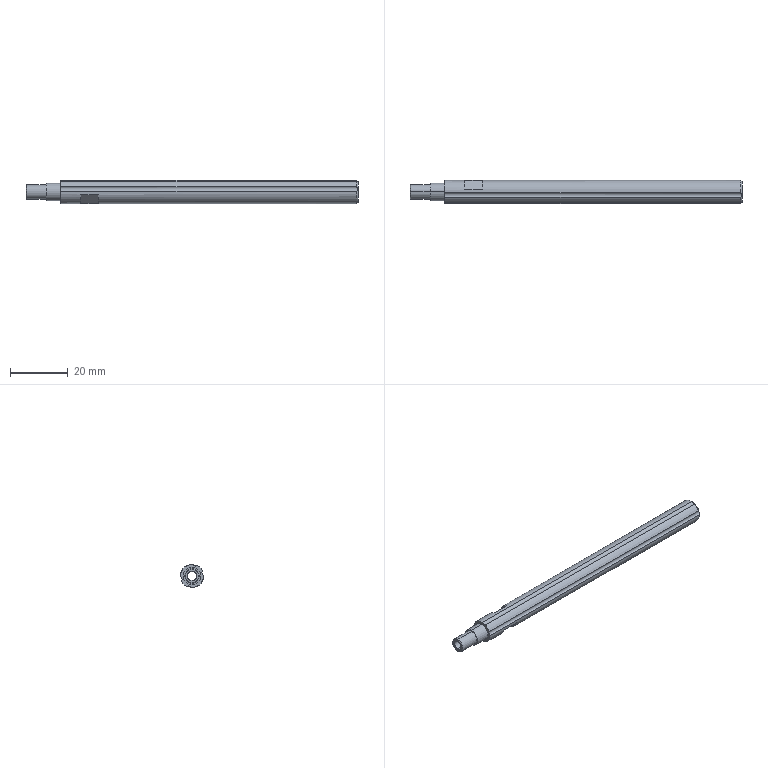Part | SolidWorks | features ICE 3, Chamfer 2, BaseBody 1, MoveFace 1 | 1 solid | 30 faces | box 115 x 8 x 8 mm | volume 4454 mm3 | cylinder 14 | plane 10 | cone 6 | commonest cylinder face diameters 2.08 x4 8 x4 3 x2 5 x2 6 x2
STEP:
#1=CARTESIAN_POINT('',(115.,0.,-3.5));
#2=VERTEX_POINT('',#1);
#3=CARTESIAN_POINT('',(115.,0.,3.5));
#4=VERTEX_POINT('',#3);
#5=CARTESIAN_POINT('',(115.,0.,0.));
#6=DIRECTION('',(1.,0.,0.));
#7=DIRECTION('',(0.,0.,-1.));
#8=AXIS2_PLACEMENT_3D('',#5,#6,#7);
#9=CIRCLE('',#8,3.5);
#10=EDGE_CURVE('',#2,#4,#9,.T.);
#11=ORIENTED_EDGE('',*,*,#10,.F.);
#12=CARTESIAN_POINT('',(114.5,0.,-4.));
#13=VERTEX_POINT('',#12);
#14=CARTESIAN_POINT('',(115.,0.,-3.5));
#15=DIRECTION('',(-0.7071,0.,-0.7071));
#16=VECTOR('',#15,1000.);
#17=LINE('',#14,#16);
#18=EDGE_CURVE('',#2,#13,#17,.T.);
#19=ORIENTED_EDGE('',*,*,#18,.T.);
#20=CARTESIAN_POINT('',(114.5,0.2928,-3.989));
#21=VERTEX_POINT('',#20);
#22=CARTESIAN_POINT('',(114.5,0.,0.));
#23=DIRECTION('',(-1.,0.,0.));
#24=DIRECTION('',(0.,0.,1.));
#25=AXIS2_PLACEMENT_3D('',#22,#23,#24);
#26=CIRCLE('',#25,4.);
#27=EDGE_CURVE('',#21,#13,#26,.T.);
#28=ORIENTED_EDGE('',*,*,#27,.F.);
#29=CARTESIAN_POINT('',(114.5,1.741,-3.601));
#30=VERTEX_POINT('',#29);
#31=CARTESIAN_POINT('',(114.5,1.741,-3.601));
#32=CARTESIAN_POINT('',(114.601,1.638,-3.539));
#33=CARTESIAN_POINT('',(114.695,1.519,-3.491));
#34=CARTESIAN_POINT('',(114.841,1.245,-3.443));
#35=CARTESIAN_POINT('',(114.89,1.087,-3.446));
#36=CARTESIAN_POINT('',(114.89,0.7827,-3.528));
#37=CARTESIAN_POINT('',(114.841,0.6442,-3.604));
#38=CARTESIAN_POINT('',(114.695,0.4305,-3.782));
#39=CARTESIAN_POINT('',(114.601,0.3513,-3.883));
#40=CARTESIAN_POINT('',(114.5,0.2928,-3.989));
#41=B_SPLINE_CURVE_WITH_KNOTS('',3,(#31,#32,#33,#34,#35,#36,#37,#38,#39,#40),.UNSPECIFIED.,.F.,.F.,(4,2,2,2,4),(0.,0.0004682,0.0009363,0.001404,0.001873),.UNSPECIFIED.);
#42=EDGE_CURVE('',#30,#21,#41,.T.);
#43=ORIENTED_EDGE('',*,*,#42,.F.);
#44=CARTESIAN_POINT('',(114.5,3.601,-1.741));
#45=VERTEX_POINT('',#44);
#46=CARTESIAN_POINT('',(114.5,0.,0.));
#47=DIRECTION('',(-1.,0.,0.));
#48=DIRECTION('',(0.,0.,1.));
#49=AXIS2_PLACEMENT_3D('',#46,#47,#48);
#50=CIRCLE('',#49,4.);
#51=EDGE_CURVE('',#45,#30,#50,.T.);
#52=ORIENTED_EDGE('',*,*,#51,.F.);
#53=CARTESIAN_POINT('',(114.5,3.989,-0.2928));
#54=VERTEX_POINT('',#53);
#55=CARTESIAN_POINT('',(114.5,3.989,-0.2928));
#56=CARTESIAN_POINT('',(114.601,3.883,-0.3512));
#57=CARTESIAN_POINT('',(114.695,3.783,-0.43));
#58=CARTESIAN_POINT('',(114.841,3.604,-0.6436));
#59=CARTESIAN_POINT('',(114.89,3.528,-0.7816));
#60=CARTESIAN_POINT('',(114.89,3.446,-1.086));
#61=CARTESIAN_POINT('',(114.841,3.443,-1.244));
#62=CARTESIAN_POINT('',(114.695,3.491,-1.518));
#63=CARTESIAN_POINT('',(114.601,3.539,-1.637));
#64=CARTESIAN_POINT('',(114.5,3.601,-1.741));
#65=B_SPLINE_CURVE_WITH_KNOTS('',3,(#55,#56,#57,#58,#59,#60,#61,#62,#63,#64),.UNSPECIFIED.,.F.,.F.,(4,2,2,2,4),(0.,0.0004682,0.0009363,0.001404,0.001873),.UNSPECIFIED.);
#66=EDGE_CURVE('',#54,#45,#65,.T.);
#67=ORIENTED_EDGE('',*,*,#66,.F.);
#68=CARTESIAN_POINT('',(114.5,0.,4.));
#69=VERTEX_POINT('',#68);
#70=CARTESIAN_POINT('',(114.5,0.,0.));
#71=DIRECTION('',(-1.,0.,0.));
#72=DIRECTION('',(0.,0.,1.));
#73=AXIS2_PLACEMENT_3D('',#70,#71,#72);
#74=CIRCLE('',#73,4.);
#75=EDGE_CURVE('',#69,#54,#74,.T.);
#76=ORIENTED_EDGE('',*,*,#75,.F.);
#77=CARTESIAN_POINT('',(115.,0.,3.5));
#78=DIRECTION('',(-0.7071,0.,0.7071));
#79=VECTOR('',#78,1000.);
#80=LINE('',#77,#79);
#81=EDGE_CURVE('',#4,#69,#80,.T.);
#82=ORIENTED_EDGE('',*,*,#81,.F.);
#83=EDGE_LOOP('',(#11,#19,#28,#43,#52,#67,#76,#82));
#84=FACE_OUTER_BOUND('',#83,.T.);
#85=CARTESIAN_POINT('',(115.,0.,0.));
#86=DIRECTION('',(-1.,0.,0.));
#87=DIRECTION('',(0.,0.,1.));
#88=AXIS2_PLACEMENT_3D('',#85,#86,#87);
#89=CONICAL_SURFACE('',#88,3.5,0.7854);
#90=ADVANCED_FACE('',(#84),#89,.T.);
#91=CARTESIAN_POINT('',(0.,0.,2.3));
#92=VERTEX_POINT('',#91);
#93=CARTESIAN_POINT('',(0.,0.,-2.3));
#94=VERTEX_POINT('',#93);
#95=CARTESIAN_POINT('',(0.,0.,0.));
#96=DIRECTION('',(-1.,0.,0.));
#97=DIRECTION('',(0.,0.,-1.));
#98=AXIS2_PLACEMENT_3D('',#95,#96,#97);
#99=CIRCLE('',#98,2.3);
#100=EDGE_CURVE('',#92,#94,#99,.T.);
#101=ORIENTED_EDGE('',*,*,#100,.F.);
#102=CARTESIAN_POINT('',(0.2,0.,2.5));
#103=VERTEX_POINT('',#102);
#104=CARTESIAN_POINT('',(0.,0.,2.3));
#105=DIRECTION('',(0.7071,0.,0.7071));
#106=VECTOR('',#105,1000.);
#107=LINE('',#104,#106);
#108=EDGE_CURVE('',#92,#103,#107,.T.);
#109=ORIENTED_EDGE('',*,*,#108,.T.);
#110=CARTESIAN_POINT('',(0.2,0.,-2.5));
#111=VERTEX_POINT('',#110);
#112=CARTESIAN_POINT('',(0.2,0.,0.));
#113=DIRECTION('',(1.,0.,0.));
#114=DIRECTION('',(0.,0.,-1.));
#115=AXIS2_PLACEMENT_3D('',#112,#113,#114);
#116=CIRCLE('',#115,2.5);
#117=EDGE_CURVE('',#111,#103,#116,.T.);
#118=ORIENTED_EDGE('',*,*,#117,.F.);
#119=CARTESIAN_POINT('',(0.,0.,-2.3));
#120=DIRECTION('',(0.7071,0.,-0.7071));
#121=VECTOR('',#120,1000.);
#122=LINE('',#119,#121);
#123=EDGE_CURVE('',#94,#111,#122,.T.);
#124=ORIENTED_EDGE('',*,*,#123,.F.);
#125=EDGE_LOOP('',(#101,#109,#118,#124));
#126=FACE_OUTER_BOUND('',#125,.T.);
#127=CARTESIAN_POINT('',(0.,0.,0.));
#128=DIRECTION('',(1.,0.,0.));
#129=DIRECTION('',(0.,0.,-1.));
#130=AXIS2_PLACEMENT_3D('',#127,#128,#129);
#131=CONICAL_SURFACE('',#130,2.3,0.7854);
#132=ADVANCED_FACE('',(#126),#131,.T.);
#133=CARTESIAN_POINT('',(7.,0.,2.5));
#134=VERTEX_POINT('',#133);
#135=CARTESIAN_POINT('',(7.,0.,-2.5));
#136=VERTEX_POINT('',#135);
#137=CARTESIAN_POINT('',(7.,0.,0.));
#138=DIRECTION('',(-1.,0.,0.));
#139=DIRECTION('',(0.,0.,1.));
#140=AXIS2_PLACEMENT_3D('',#137,#138,#139);
#141=CIRCLE('',#140,2.5);
#142=EDGE_CURVE('',#134,#136,#141,.T.);
#143=ORIENTED_EDGE('',*,*,#142,.T.);
#144=CARTESIAN_POINT('',(7.,0.,-2.5));
#145=DIRECTION('',(-1.,0.,0.));
#146=VECTOR('',#145,1000.);
#147=LINE('',#144,#146);
#148=EDGE_CURVE('',#136,#111,#147,.T.);
#149=ORIENTED_EDGE('',*,*,#148,.T.);
#150=ORIENTED_EDGE('',*,*,#117,.T.);
#151=CARTESIAN_POINT('',(7.,0.,2.5));
#152=DIRECTION('',(-1.,0.,0.));
#153=VECTOR('',#152,1000.);
#154=LINE('',#151,#153);
#155=EDGE_CURVE('',#134,#103,#154,.T.);
#156=ORIENTED_EDGE('',*,*,#155,.F.);
#157=EDGE_LOOP('',(#143,#149,#150,#156));
#158=FACE_OUTER_BOUND('',#157,.T.);
#159=CARTESIAN_POINT('',(7.,0.,0.));
#160=DIRECTION('',(-1.,0.,0.));
#161=DIRECTION('',(0.,0.,1.));
#162=AXIS2_PLACEMENT_3D('',#159,#160,#161);
#163=CYLINDRICAL_SURFACE('',#162,2.5);
#164=ADVANCED_FACE('',(#158),#163,.T.);
#165=CARTESIAN_POINT('',(12.,0.,3.));
#166=VERTEX_POINT('',#165);
#167=CARTESIAN_POINT('',(12.,0.,-3.));
#168=VERTEX_POINT('',#167);
#169=CARTESIAN_POINT('',(12.,0.,0.));
#170=DIRECTION('',(-1.,0.,0.));
#171=DIRECTION('',(0.,0.,1.));
#172=AXIS2_PLACEMENT_3D('',#169,#170,#171);
#173=CIRCLE('',#172,3.);
#174=EDGE_CURVE('',#166,#168,#173,.T.);
#175=ORIENTED_EDGE('',*,*,#174,.T.);
#176=CARTESIAN_POINT('',(7.,0.,-3.));
#177=VERTEX_POINT('',#176);
#178=CARTESIAN_POINT('',(12.,0.,-3.));
#179=DIRECTION('',(-1.,0.,0.));
#180=VECTOR('',#179,1000.);
#181=LINE('',#178,#180);
#182=EDGE_CURVE('',#168,#177,#181,.T.);
#183=ORIENTED_EDGE('',*,*,#182,.T.);
#184=CARTESIAN_POINT('',(7.,0.,3.));
#185=VERTEX_POINT('',#184);
#186=CARTESIAN_POINT('',(7.,0.,0.));
#187=DIRECTION('',(1.,0.,0.));
#188=DIRECTION('',(0.,0.,1.));
#189=AXIS2_PLACEMENT_3D('',#186,#187,#188);
#190=CIRCLE('',#189,3.);
#191=EDGE_CURVE('',#177,#185,#190,.T.);
#192=ORIENTED_EDGE('',*,*,#191,.T.);
#193=CARTESIAN_POINT('',(12.,0.,3.));
#194=DIRECTION('',(-1.,0.,0.));
#195=VECTOR('',#194,1000.);
#196=LINE('',#193,#195);
#197=EDGE_CURVE('',#166,#185,#196,.T.);
#198=ORIENTED_EDGE('',*,*,#197,.F.);
#199=EDGE_LOOP('',(#175,#183,#192,#198));
#200=FACE_OUTER_BOUND('',#199,.T.);
#201=CARTESIAN_POINT('',(12.,0.,0.));
#202=DIRECTION('',(-1.,0.,0.));
#203=DIRECTION('',(0.,0.,1.));
#204=AXIS2_PLACEMENT_3D('',#201,#202,#203);
#205=CYLINDRICAL_SURFACE('',#204,3.);
#206=ADVANCED_FACE('',(#200),#205,.T.);
#207=CARTESIAN_POINT('',(12.,0.2928,-3.989));
#208=VERTEX_POINT('',#207);
#209=CARTESIAN_POINT('',(90.,0.2928,-3.989));
#210=DIRECTION('',(-1.,0.,0.));
#211=VECTOR('',#210,1000.);
#212=LINE('',#209,#211);
#213=EDGE_CURVE('',#21,#208,#212,.T.);
#214=ORIENTED_EDGE('',*,*,#213,.F.);
#215=ORIENTED_EDGE('',*,*,#27,.T.);
#216=CARTESIAN_POINT('',(114.5,-3.989,0.2928));
#217=VERTEX_POINT('',#216);
#218=CARTESIAN_POINT('',(114.5,0.,0.));
#219=DIRECTION('',(-1.,0.,0.));
#220=DIRECTION('',(0.,0.,1.));
#221=AXIS2_PLACEMENT_3D('',#218,#219,#220);
#222=CIRCLE('',#221,4.);
#223=EDGE_CURVE('',#13,#217,#222,.T.);
#224=ORIENTED_EDGE('',*,*,#223,.T.);
#225=CARTESIAN_POINT('',(12.,-3.989,0.2928));
#226=VERTEX_POINT('',#225);
#227=CARTESIAN_POINT('',(90.,-3.989,0.2928));
#228=DIRECTION('',(-1.,0.,0.));
#229=VECTOR('',#228,1000.);
#230=LINE('',#227,#229);
#231=EDGE_CURVE('',#217,#226,#230,.T.);
#232=ORIENTED_EDGE('',*,*,#231,.T.);
#233=CARTESIAN_POINT('',(12.,0.,0.));
#234=DIRECTION('',(1.,0.,0.));
#235=DIRECTION('',(0.,0.,1.));
#236=AXIS2_PLACEMENT_3D('',#233,#234,#235);
#237=CIRCLE('',#236,4.);
#238=EDGE_CURVE('',#226,#208,#237,.T.);
#239=ORIENTED_EDGE('',*,*,#238,.T.);
#240=EDGE_LOOP('',(#214,#215,#224,#232,#239));
#241=FACE_OUTER_BOUND('',#240,.T.);
#242=CARTESIAN_POINT('',(19.,-0.9142,-3.894));
#243=VERTEX_POINT('',#242);
#244=CARTESIAN_POINT('',(25.,-0.9142,-3.894));
#245=VERTEX_POINT('',#244);
#246=CARTESIAN_POINT('',(90.,-0.9142,-3.894));
#247=DIRECTION('',(1.,0.,0.));
#248=VECTOR('',#247,1000.);
#249=LINE('',#246,#248);
#250=EDGE_CURVE('',#243,#245,#249,.T.);
#251=ORIENTED_EDGE('',*,*,#250,.F.);
#252=CARTESIAN_POINT('',(19.,-3.894,-0.9142));
#253=VERTEX_POINT('',#252);
#254=CARTESIAN_POINT('',(19.,0.,0.));
#255=DIRECTION('',(-1.,0.,0.));
#256=DIRECTION('',(0.,0.,-1.));
#257=AXIS2_PLACEMENT_3D('',#254,#255,#256);
#258=CIRCLE('',#257,4.);
#259=EDGE_CURVE('',#243,#253,#258,.T.);
#260=ORIENTED_EDGE('',*,*,#259,.T.);
#261=CARTESIAN_POINT('',(25.,-3.894,-0.9142));
#262=VERTEX_POINT('',#261);
#263=CARTESIAN_POINT('',(90.,-3.894,-0.9142));
#264=DIRECTION('',(-1.,0.,0.));
#265=VECTOR('',#264,1000.);
#266=LINE('',#263,#265);
#267=EDGE_CURVE('',#262,#253,#266,.T.);
#268=ORIENTED_EDGE('',*,*,#267,.F.);
#269=CARTESIAN_POINT('',(25.,0.,0.));
#270=DIRECTION('',(-1.,0.,0.));
#271=DIRECTION('',(0.,0.,-1.));
#272=AXIS2_PLACEMENT_3D('',#269,#270,#271);
#273=CIRCLE('',#272,4.);
#274=EDGE_CURVE('',#245,#262,#273,.T.);
#275=ORIENTED_EDGE('',*,*,#274,.F.);
#276=EDGE_LOOP('',(#251,#260,#268,#275));
#277=FACE_BOUND('',#276,.T.);
#278=CARTESIAN_POINT('',(90.,0.,0.));
#279=DIRECTION('',(-1.,0.,0.));
#280=DIRECTION('',(0.,0.7071,0.7071));
#281=AXIS2_PLACEMENT_3D('',#278,#279,#280);
#282=CYLINDRICAL_SURFACE('',#281,4.);
#283=ADVANCED_FACE('',(#241,#277),#282,.T.);
#284=CARTESIAN_POINT('',(114.5,-0.2928,3.989));
#285=VERTEX_POINT('',#284);
#286=CARTESIAN_POINT('',(12.,-0.2928,3.989));
#287=VERTEX_POINT('',#286);
#288=CARTESIAN_POINT('',(90.,-0.2928,3.989));
#289=DIRECTION('',(-1.,0.,0.));
#290=VECTOR('',#289,1000.);
#291=LINE('',#288,#290);
#292=EDGE_CURVE('',#285,#287,#291,.T.);
#293=ORIENTED_EDGE('',*,*,#292,.F.);
#294=CARTESIAN_POINT('',(114.5,0.,0.));
#295=DIRECTION('',(-1.,0.,0.));
#296=DIRECTION('',(0.,0.,1.));
#297=AXIS2_PLACEMENT_3D('',#294,#295,#296);
#298=CIRCLE('',#297,4.);
#299=EDGE_CURVE('',#285,#69,#298,.T.);
#300=ORIENTED_EDGE('',*,*,#299,.T.);
#301=ORIENTED_EDGE('',*,*,#75,.T.);
#302=CARTESIAN_POINT('',(12.,3.989,-0.2928));
#303=VERTEX_POINT('',#302);
#304=CARTESIAN_POINT('',(90.,3.989,-0.2928));
#305=DIRECTION('',(-1.,0.,0.));
#306=VECTOR('',#305,1000.);
#307=LINE('',#304,#306);
#308=EDGE_CURVE('',#54,#303,#307,.T.);
#309=ORIENTED_EDGE('',*,*,#308,.T.);
#310=CARTESIAN_POINT('',(12.,0.,0.));
#311=DIRECTION('',(1.,0.,0.));
#312=DIRECTION('',(0.,0.,1.));
#313=AXIS2_PLACEMENT_3D('',#310,#311,#312);
#314=CIRCLE('',#313,4.);
#315=EDGE_CURVE('',#303,#287,#314,.T.);
#316=ORIENTED_EDGE('',*,*,#315,.T.);
#317=EDGE_LOOP('',(#293,#300,#301,#309,#316));
#318=FACE_OUTER_BOUND('',#317,.T.);
#319=CARTESIAN_POINT('',(19.,0.9142,3.894));
#320=VERTEX_POINT('',#319);
#321=CARTESIAN_POINT('',(25.,0.9142,3.894));
#322=VERTEX_POINT('',#321);
#323=CARTESIAN_POINT('',(90.,0.9142,3.894));
#324=DIRECTION('',(1.,0.,0.));
#325=VECTOR('',#324,1000.);
#326=LINE('',#323,#325);
#327=EDGE_CURVE('',#320,#322,#326,.T.);
#328=ORIENTED_EDGE('',*,*,#327,.F.);
#329=CARTESIAN_POINT('',(19.,3.894,0.9142));
#330=VERTEX_POINT('',#329);
#331=CARTESIAN_POINT('',(19.,0.,0.));
#332=DIRECTION('',(-1.,0.,0.));
#333=DIRECTION('',(0.,0.,-1.));
#334=AXIS2_PLACEMENT_3D('',#331,#332,#333);
#335=CIRCLE('',#334,4.);
#336=EDGE_CURVE('',#320,#330,#335,.T.);
#337=ORIENTED_EDGE('',*,*,#336,.T.);
#338=CARTESIAN_POINT('',(25.,3.894,0.9142));
#339=VERTEX_POINT('',#338);
#340=CARTESIAN_POINT('',(90.,3.894,0.9142));
#341=DIRECTION('',(-1.,0.,0.));
#342=VECTOR('',#341,1000.);
#343=LINE('',#340,#342);
#344=EDGE_CURVE('',#339,#330,#343,.T.);
#345=ORIENTED_EDGE('',*,*,#344,.F.);
#346=CARTESIAN_POINT('',(25.,0.,0.));
#347=DIRECTION('',(-1.,0.,0.));
#348=DIRECTION('',(0.,0.,-1.));
#349=AXIS2_PLACEMENT_3D('',#346,#347,#348);
#350=CIRCLE('',#349,4.);
#351=EDGE_CURVE('',#322,#339,#350,.T.);
#352=ORIENTED_EDGE('',*,*,#351,.F.);
#353=EDGE_LOOP('',(#328,#337,#345,#352));
#354=FACE_BOUND('',#353,.T.);
#355=CARTESIAN_POINT('',(90.,0.,0.));
#356=DIRECTION('',(-1.,0.,0.));
#357=DIRECTION('',(0.,-0.7071,-0.7071));
#358=AXIS2_PLACEMENT_3D('',#355,#356,#357);
#359=CYLINDRICAL_SURFACE('',#358,4.);
#360=ADVANCED_FACE('',(#318,#354),#359,.T.);
#361=CARTESIAN_POINT('',(0.,0.,-1.7));
#362=VERTEX_POINT('',#361);
#363=CARTESIAN_POINT('',(0.,0.,1.7));
#364=VERTEX_POINT('',#363);
#365=CARTESIAN_POINT('',(0.,0.,0.));
#366=DIRECTION('',(1.,0.,0.));
#367=DIRECTION('',(0.,0.,-1.));
#368=AXIS2_PLACEMENT_3D('',#365,#366,#367);
#369=CIRCLE('',#368,1.7);
#370=EDGE_CURVE('',#362,#364,#369,.T.);
#371=ORIENTED_EDGE('',*,*,#370,.T.);
#372=CARTESIAN_POINT('',(0.,0.,0.));
#373=DIRECTION('',(1.,0.,0.));
#374=DIRECTION('',(0.,0.,-1.));
#375=AXIS2_PLACEMENT_3D('',#372,#373,#374);
#376=CIRCLE('',#375,1.7);
#377=EDGE_CURVE('',#364,#362,#376,.T.);
#378=ORIENTED_EDGE('',*,*,#377,.T.);
#379=EDGE_LOOP('',(#371,#378));
#380=FACE_BOUND('',#379,.T.);
#381=CARTESIAN_POINT('',(0.,0.,0.));
#382=DIRECTION('',(-1.,0.,0.));
#383=DIRECTION('',(0.,0.,-1.));
#384=AXIS2_PLACEMENT_3D('',#381,#382,#383);
#385=CIRCLE('',#384,2.3);
#386=EDGE_CURVE('',#94,#92,#385,.T.);
#387=ORIENTED_EDGE('',*,*,#386,.T.);
#388=ORIENTED_EDGE('',*,*,#100,.T.);
#389=EDGE_LOOP('',(#387,#388));
#390=FACE_OUTER_BOUND('',#389,.T.);
#391=CARTESIAN_POINT('',(0.,2.246,-0.6018));
#392=DIRECTION('',(1.,0.,0.));
#393=DIRECTION('',(0.,0.,-1.));
#394=AXIS2_PLACEMENT_3D('',#391,#392,#393);
#395=PLANE('',#394);
#396=ADVANCED_FACE('',(#380,#390),#395,.F.);
#397=ORIENTED_EDGE('',*,*,#182,.F.);
#398=CARTESIAN_POINT('',(12.,0.,0.));
#399=DIRECTION('',(-1.,0.,0.));
#400=DIRECTION('',(0.,0.,1.));
#401=AXIS2_PLACEMENT_3D('',#398,#399,#400);
#402=CIRCLE('',#401,3.);
#403=EDGE_CURVE('',#168,#166,#402,.T.);
#404=ORIENTED_EDGE('',*,*,#403,.T.);
#405=ORIENTED_EDGE('',*,*,#197,.T.);
#406=CARTESIAN_POINT('',(7.,0.,0.));
#407=DIRECTION('',(1.,0.,0.));
#408=DIRECTION('',(0.,0.,1.));
#409=AXIS2_PLACEMENT_3D('',#406,#407,#408);
#410=CIRCLE('',#409,3.);
#411=EDGE_CURVE('',#185,#177,#410,.T.);
#412=ORIENTED_EDGE('',*,*,#411,.T.);
#413=EDGE_LOOP('',(#397,#404,#405,#412));
#414=FACE_OUTER_BOUND('',#413,.T.);
#415=CARTESIAN_POINT('',(12.,0.,0.));
#416=DIRECTION('',(-1.,0.,0.));
#417=DIRECTION('',(0.,0.,1.));
#418=AXIS2_PLACEMENT_3D('',#415,#416,#417);
#419=CYLINDRICAL_SURFACE('',#418,3.);
#420=ADVANCED_FACE('',(#414),#419,.T.);
#421=ORIENTED_EDGE('',*,*,#308,.F.);
#422=ORIENTED_EDGE('',*,*,#66,.T.);
#423=CARTESIAN_POINT('',(12.,3.601,-1.741));
#424=VERTEX_POINT('',#423);
#425=CARTESIAN_POINT('',(90.,3.601,-1.741));
#426=DIRECTION('',(-1.,0.,0.));
#427=VECTOR('',#426,1000.);
#428=LINE('',#425,#427);
#429=EDGE_CURVE('',#45,#424,#428,.T.);
#430=ORIENTED_EDGE('',*,*,#429,.T.);
#431=CARTESIAN_POINT('',(12.,4.492,-1.204));
#432=DIRECTION('',(1.,0.,0.));
#433=DIRECTION('',(0.,0.,1.));
#434=AXIS2_PLACEMENT_3D('',#431,#432,#433);
#435=CIRCLE('',#434,1.04);
#436=EDGE_CURVE('',#303,#424,#435,.T.);
#437=ORIENTED_EDGE('',*,*,#436,.F.);
#438=EDGE_LOOP('',(#421,#422,#430,#437));
#439=FACE_OUTER_BOUND('',#438,.T.);
#440=CARTESIAN_POINT('',(90.,4.492,-1.204));
#441=DIRECTION('',(-1.,0.,0.));
#442=DIRECTION('',(0.,0.9659,-0.2588));
#443=AXIS2_PLACEMENT_3D('',#440,#441,#442);
#444=CYLINDRICAL_SURFACE('',#443,1.04);
#445=ADVANCED_FACE('',(#439),#444,.F.);
#446=ORIENTED_EDGE('',*,*,#429,.F.);
#447=ORIENTED_EDGE('',*,*,#51,.T.);
#448=CARTESIAN_POINT('',(12.,1.741,-3.601));
#449=VERTEX_POINT('',#448);
#450=CARTESIAN_POINT('',(90.,1.741,-3.601));
#451=DIRECTION('',(-1.,0.,0.));
#452=VECTOR('',#451,1000.);
#453=LINE('',#450,#452);
#454=EDGE_CURVE('',#30,#449,#453,.T.);
#455=ORIENTED_EDGE('',*,*,#454,.T.);
#456=CARTESIAN_POINT('',(12.,0.,0.));
#457=DIRECTION('',(1.,0.,0.));
#458=DIRECTION('',(0.,0.,1.));
#459=AXIS2_PLACEMENT_3D('',#456,#457,#458);
#460=CIRCLE('',#459,4.);
#461=EDGE_CURVE('',#449,#424,#460,.T.);
#462=ORIENTED_EDGE('',*,*,#461,.T.);
#463=EDGE_LOOP('',(#446,#447,#455,#462));
#464=FACE_OUTER_BOUND('',#463,.T.);
#465=CARTESIAN_POINT('',(90.,0.,0.));
#466=DIRECTION('',(-1.,0.,0.));
#467=DIRECTION('',(0.,-0.7071,0.7071));
#468=AXIS2_PLACEMENT_3D('',#465,#466,#467);
#469=CYLINDRICAL_SURFACE('',#468,4.);
#470=ADVANCED_FACE('',(#464),#469,.T.);
#471=ORIENTED_EDGE('',*,*,#454,.F.);
#472=ORIENTED_EDGE('',*,*,#42,.T.);
#473=ORIENTED_EDGE('',*,*,#213,.T.);
#474=CARTESIAN_POINT('',(12.,1.204,-4.492));
#475=DIRECTION('',(1.,0.,0.));
#476=DIRECTION('',(0.,0.,1.));
#477=AXIS2_PLACEMENT_3D('',#474,#475,#476);
#478=CIRCLE('',#477,1.04);
#479=EDGE_CURVE('',#449,#208,#478,.T.);
#480=ORIENTED_EDGE('',*,*,#479,.F.);
#481=EDGE_LOOP('',(#471,#472,#473,#480));
#482=FACE_OUTER_BOUND('',#481,.T.);
#483=CARTESIAN_POINT('',(90.,1.204,-4.492));
#484=DIRECTION('',(-1.,0.,0.));
#485=DIRECTION('',(0.,0.2588,-0.9659));
#486=AXIS2_PLACEMENT_3D('',#483,#484,#485);
#487=CYLINDRICAL_SURFACE('',#486,1.04);
#488=ADVANCED_FACE('',(#482),#487,.F.);
#489=ORIENTED_EDGE('',*,*,#231,.F.);
#490=CARTESIAN_POINT('',(114.5,-3.601,1.741));
#491=VERTEX_POINT('',#490);
#492=CARTESIAN_POINT('',(114.5,-3.989,0.2928));
#493=CARTESIAN_POINT('',(114.601,-3.883,0.3512));
#494=CARTESIAN_POINT('',(114.695,-3.783,0.43));
#495=CARTESIAN_POINT('',(114.841,-3.604,0.6436));
#496=CARTESIAN_POINT('',(114.89,-3.528,0.7816));
#497=CARTESIAN_POINT('',(114.89,-3.446,1.086));
#498=CARTESIAN_POINT('',(114.841,-3.443,1.244));
#499=CARTESIAN_POINT('',(114.695,-3.491,1.518));
#500=CARTESIAN_POINT('',(114.601,-3.539,1.637));
#501=CARTESIAN_POINT('',(114.5,-3.601,1.741));
#502=B_SPLINE_CURVE_WITH_KNOTS('',3,(#492,#493,#494,#495,#496,#497,#498,#499,#500,#501),.UNSPECIFIED.,.F.,.F.,(4,2,2,2,4),(0.,0.0004682,0.0009363,0.001404,0.001873),.UNSPECIFIED.);
#503=EDGE_CURVE('',#217,#491,#502,.T.);
#504=ORIENTED_EDGE('',*,*,#503,.T.);
#505=CARTESIAN_POINT('',(12.,-3.601,1.741));
#506=VERTEX_POINT('',#505);
#507=CARTESIAN_POINT('',(90.,-3.601,1.741));
#508=DIRECTION('',(-1.,0.,0.));
#509=VECTOR('',#508,1000.);
#510=LINE('',#507,#509);
#511=EDGE_CURVE('',#491,#506,#510,.T.);
#512=ORIENTED_EDGE('',*,*,#511,.T.);
#513=CARTESIAN_POINT('',(12.,-4.492,1.204));
#514=DIRECTION('',(1.,0.,0.));
#515=DIRECTION('',(0.,0.,1.));
#516=AXIS2_PLACEMENT_3D('',#513,#514,#515);
#517=CIRCLE('',#516,1.04);
#518=EDGE_CURVE('',#226,#506,#517,.T.);
#519=ORIENTED_EDGE('',*,*,#518,.F.);
#520=EDGE_LOOP('',(#489,#504,#512,#519));
#521=FACE_OUTER_BOUND('',#520,.T.);
#522=CARTESIAN_POINT('',(90.,-4.492,1.204));
#523=DIRECTION('',(-1.,0.,0.));
#524=DIRECTION('',(0.,-0.9659,0.2588));
#525=AXIS2_PLACEMENT_3D('',#522,#523,#524);
#526=CYLINDRICAL_SURFACE('',#525,1.04);
#527=ADVANCED_FACE('',(#521),#526,.F.);
#528=ORIENTED_EDGE('',*,*,#511,.F.);
#529=CARTESIAN_POINT('',(114.5,-1.741,3.601));
#530=VERTEX_POINT('',#529);
#531=CARTESIAN_POINT('',(114.5,0.,0.));
#532=DIRECTION('',(-1.,0.,0.));
#533=DIRECTION('',(0.,0.,-1.));
#534=AXIS2_PLACEMENT_3D('',#531,#532,#533);
#535=CIRCLE('',#534,4.);
#536=EDGE_CURVE('',#491,#530,#535,.T.);
#537=ORIENTED_EDGE('',*,*,#536,.T.);
#538=CARTESIAN_POINT('',(12.,-1.741,3.601));
#539=VERTEX_POINT('',#538);
#540=CARTESIAN_POINT('',(90.,-1.741,3.601));
#541=DIRECTION('',(-1.,0.,0.));
#542=VECTOR('',#541,1000.);
#543=LINE('',#540,#542);
#544=EDGE_CURVE('',#530,#539,#543,.T.);
#545=ORIENTED_EDGE('',*,*,#544,.T.);
#546=CARTESIAN_POINT('',(12.,0.,0.));
#547=DIRECTION('',(1.,0.,0.));
#548=DIRECTION('',(0.,0.,1.));
#549=AXIS2_PLACEMENT_3D('',#546,#547,#548);
#550=CIRCLE('',#549,4.);
#551=EDGE_CURVE('',#539,#506,#550,.T.);
#552=ORIENTED_EDGE('',*,*,#551,.T.);
#553=EDGE_LOOP('',(#528,#537,#545,#552));
#554=FACE_OUTER_BOUND('',#553,.T.);
#555=CARTESIAN_POINT('',(90.,0.,0.));
#556=DIRECTION('',(-1.,0.,0.));
#557=DIRECTION('',(0.,0.7071,-0.7071));
#558=AXIS2_PLACEMENT_3D('',#555,#556,#557);
#559=CYLINDRICAL_SURFACE('',#558,4.);
#560=ADVANCED_FACE('',(#554),#559,.T.);
#561=ORIENTED_EDGE('',*,*,#544,.F.);
#562=CARTESIAN_POINT('',(114.5,-1.741,3.601));
#563=CARTESIAN_POINT('',(114.601,-1.638,3.539));
#564=CARTESIAN_POINT('',(114.695,-1.519,3.491));
#565=CARTESIAN_POINT('',(114.841,-1.245,3.443));
#566=CARTESIAN_POINT('',(114.89,-1.087,3.446));
#567=CARTESIAN_POINT('',(114.89,-0.7827,3.528));
#568=CARTESIAN_POINT('',(114.841,-0.6442,3.604));
#569=CARTESIAN_POINT('',(114.695,-0.4305,3.782));
#570=CARTESIAN_POINT('',(114.601,-0.3513,3.883));
#571=CARTESIAN_POINT('',(114.5,-0.2928,3.989));
#572=B_SPLINE_CURVE_WITH_KNOTS('',3,(#562,#563,#564,#565,#566,#567,#568,#569,#570,#571),.UNSPECIFIED.,.F.,.F.,(4,2,2,2,4),(0.,0.0004682,0.0009363,0.001404,0.001873),.UNSPECIFIED.);
#573=EDGE_CURVE('',#530,#285,#572,.T.);
#574=ORIENTED_EDGE('',*,*,#573,.T.);
#575=ORIENTED_EDGE('',*,*,#292,.T.);
#576=CARTESIAN_POINT('',(12.,-1.204,4.492));
#577=DIRECTION('',(1.,0.,0.));
#578=DIRECTION('',(0.,0.,1.));
#579=AXIS2_PLACEMENT_3D('',#576,#577,#578);
#580=CIRCLE('',#579,1.04);
#581=EDGE_CURVE('',#539,#287,#580,.T.);
#582=ORIENTED_EDGE('',*,*,#581,.F.);
#583=EDGE_LOOP('',(#561,#574,#575,#582));
#584=FACE_OUTER_BOUND('',#583,.T.);
#585=CARTESIAN_POINT('',(90.,-1.204,4.492));
#586=DIRECTION('',(-1.,0.,0.));
#587=DIRECTION('',(0.,-0.2588,0.9659));
#588=AXIS2_PLACEMENT_3D('',#585,#586,#587);
#589=CYLINDRICAL_SURFACE('',#588,1.04);
#590=ADVANCED_FACE('',(#584),#589,.F.);
#591=CARTESIAN_POINT('',(115.,0.,0.));
#592=DIRECTION('',(1.,0.,0.));
#593=DIRECTION('',(0.,0.,-1.));
#594=AXIS2_PLACEMENT_3D('',#591,#592,#593);
#595=CIRCLE('',#594,3.5);
#596=EDGE_CURVE('',#4,#2,#595,.T.);
#597=ORIENTED_EDGE('',*,*,#596,.T.);
#598=ORIENTED_EDGE('',*,*,#10,.T.);
#599=EDGE_LOOP('',(#597,#598));
#600=FACE_OUTER_BOUND('',#599,.T.);
#601=CARTESIAN_POINT('',(115.,0.,1.5));
#602=VERTEX_POINT('',#601);
#603=CARTESIAN_POINT('',(115.,0.,-1.5));
#604=VERTEX_POINT('',#603);
#605=CARTESIAN_POINT('',(115.,0.,0.));
#606=DIRECTION('',(1.,0.,0.));
#607=DIRECTION('',(0.,0.,-1.));
#608=AXIS2_PLACEMENT_3D('',#605,#606,#607);
#609=CIRCLE('',#608,1.5);
#610=EDGE_CURVE('',#602,#604,#609,.T.);
#611=ORIENTED_EDGE('',*,*,#610,.F.);
#612=CARTESIAN_POINT('',(115.,0.,0.));
#613=DIRECTION('',(1.,0.,0.));
#614=DIRECTION('',(0.,0.,-1.));
#615=AXIS2_PLACEMENT_3D('',#612,#613,#614);
#616=CIRCLE('',#615,1.5);
#617=EDGE_CURVE('',#604,#602,#616,.T.);
#618=ORIENTED_EDGE('',*,*,#617,.F.);
#619=EDGE_LOOP('',(#611,#618));
#620=FACE_BOUND('',#619,.T.);
#621=CARTESIAN_POINT('',(115.,2.246,-0.6018));
#622=DIRECTION('',(1.,0.,0.));
#623=DIRECTION('',(0.,0.,-1.));
#624=AXIS2_PLACEMENT_3D('',#621,#622,#623);
#625=PLANE('',#624);
#626=ADVANCED_FACE('',(#600,#620),#625,.T.);
#627=CARTESIAN_POINT('',(0.2,0.,1.5));
#628=VERTEX_POINT('',#627);
#629=CARTESIAN_POINT('',(90.,0.,1.5));
#630=DIRECTION('',(-1.,0.,0.));
#631=VECTOR('',#630,1000.);
#632=LINE('',#629,#631);
#633=EDGE_CURVE('',#602,#628,#632,.T.);
#634=ORIENTED_EDGE('',*,*,#633,.T.);
#635=CARTESIAN_POINT('',(0.2,0.,-1.5));
#636=VERTEX_POINT('',#635);
#637=CARTESIAN_POINT('',(0.2,0.,0.));
#638=DIRECTION('',(-1.,0.,0.));
#639=DIRECTION('',(0.,0.,-1.));
#640=AXIS2_PLACEMENT_3D('',#637,#638,#639);
#641=CIRCLE('',#640,1.5);
#642=EDGE_CURVE('',#628,#636,#641,.T.);
#643=ORIENTED_EDGE('',*,*,#642,.T.);
#644=CARTESIAN_POINT('',(90.,0.,-1.5));
#645=DIRECTION('',(-1.,0.,0.));
#646=VECTOR('',#645,1000.);
#647=LINE('',#644,#646);
#648=EDGE_CURVE('',#604,#636,#647,.T.);
#649=ORIENTED_EDGE('',*,*,#648,.F.);
#650=ORIENTED_EDGE('',*,*,#617,.T.);
#651=EDGE_LOOP('',(#634,#643,#649,#650));
#652=FACE_OUTER_BOUND('',#651,.T.);
#653=CARTESIAN_POINT('',(90.,0.,0.));
#654=DIRECTION('',(-1.,0.,0.));
#655=DIRECTION('',(0.,-1.,0.));
#656=AXIS2_PLACEMENT_3D('',#653,#654,#655);
#657=CYLINDRICAL_SURFACE('',#656,1.5);
#658=ADVANCED_FACE('',(#652),#657,.F.);
#659=ORIENTED_EDGE('',*,*,#648,.T.);
#660=CARTESIAN_POINT('',(0.2,0.,0.));
#661=DIRECTION('',(-1.,0.,0.));
#662=DIRECTION('',(0.,0.,-1.));
#663=AXIS2_PLACEMENT_3D('',#660,#661,#662);
#664=CIRCLE('',#663,1.5);
#665=EDGE_CURVE('',#636,#628,#664,.T.);
#666=ORIENTED_EDGE('',*,*,#665,.T.);
#667=ORIENTED_EDGE('',*,*,#633,.F.);
#668=ORIENTED_EDGE('',*,*,#610,.T.);
#669=EDGE_LOOP('',(#659,#666,#667,#668));
#670=FACE_OUTER_BOUND('',#669,.T.);
#671=CARTESIAN_POINT('',(90.,0.,0.));
#672=DIRECTION('',(-1.,0.,0.));
#673=DIRECTION('',(0.,1.,0.));
#674=AXIS2_PLACEMENT_3D('',#671,#672,#673);
#675=CYLINDRICAL_SURFACE('',#674,1.5);
#676=ADVANCED_FACE('',(#670),#675,.F.);
#677=ORIENTED_EDGE('',*,*,#174,.F.);
#678=ORIENTED_EDGE('',*,*,#403,.F.);
#679=EDGE_LOOP('',(#677,#678));
#680=FACE_BOUND('',#679,.T.);
#681=ORIENTED_EDGE('',*,*,#436,.T.);
#682=ORIENTED_EDGE('',*,*,#461,.F.);
#683=ORIENTED_EDGE('',*,*,#479,.T.);
#684=ORIENTED_EDGE('',*,*,#238,.F.);
#685=ORIENTED_EDGE('',*,*,#518,.T.);
#686=ORIENTED_EDGE('',*,*,#551,.F.);
#687=ORIENTED_EDGE('',*,*,#581,.T.);
#688=ORIENTED_EDGE('',*,*,#315,.F.);
#689=EDGE_LOOP('',(#681,#682,#683,#684,#685,#686,#687,#688));
#690=FACE_OUTER_BOUND('',#689,.T.);
#691=CARTESIAN_POINT('',(12.,0.,0.));
#692=DIRECTION('',(-1.,0.,0.));
#693=DIRECTION('',(0.,0.,1.));
#694=AXIS2_PLACEMENT_3D('',#691,#692,#693);
#695=PLANE('',#694);
#696=ADVANCED_FACE('',(#680,#690),#695,.T.);
#697=ORIENTED_EDGE('',*,*,#411,.F.);
#698=ORIENTED_EDGE('',*,*,#191,.F.);
#699=EDGE_LOOP('',(#697,#698));
#700=FACE_OUTER_BOUND('',#699,.T.);
#701=ORIENTED_EDGE('',*,*,#142,.F.);
#702=CARTESIAN_POINT('',(7.,0.,0.));
#703=DIRECTION('',(-1.,0.,0.));
#704=DIRECTION('',(0.,0.,1.));
#705=AXIS2_PLACEMENT_3D('',#702,#703,#704);
#706=CIRCLE('',#705,2.5);
#707=EDGE_CURVE('',#136,#134,#706,.T.);
#708=ORIENTED_EDGE('',*,*,#707,.F.);
#709=EDGE_LOOP('',(#701,#708));
#710=FACE_BOUND('',#709,.T.);
#711=CARTESIAN_POINT('',(7.,0.,0.));
#712=DIRECTION('',(-1.,0.,0.));
#713=DIRECTION('',(0.,0.,1.));
#714=AXIS2_PLACEMENT_3D('',#711,#712,#713);
#715=PLANE('',#714);
#716=ADVANCED_FACE('',(#700,#710),#715,.T.);
#717=ORIENTED_EDGE('',*,*,#148,.F.);
#718=ORIENTED_EDGE('',*,*,#707,.T.);
#719=ORIENTED_EDGE('',*,*,#155,.T.);
#720=CARTESIAN_POINT('',(0.2,0.,0.));
#721=DIRECTION('',(1.,0.,0.));
#722=DIRECTION('',(0.,0.,-1.));
#723=AXIS2_PLACEMENT_3D('',#720,#721,#722);
#724=CIRCLE('',#723,2.5);
#725=EDGE_CURVE('',#103,#111,#724,.T.);
#726=ORIENTED_EDGE('',*,*,#725,.T.);
#727=EDGE_LOOP('',(#717,#718,#719,#726));
#728=FACE_OUTER_BOUND('',#727,.T.);
#729=CARTESIAN_POINT('',(7.,0.,0.));
#730=DIRECTION('',(-1.,0.,0.));
#731=DIRECTION('',(0.,0.,1.));
#732=AXIS2_PLACEMENT_3D('',#729,#730,#731);
#733=CYLINDRICAL_SURFACE('',#732,2.5);
#734=ADVANCED_FACE('',(#728),#733,.T.);
#735=CARTESIAN_POINT('',(0.2,0.,-1.5));
#736=DIRECTION('',(-0.7071,0.,-0.7071));
#737=VECTOR('',#736,1000.);
#738=LINE('',#735,#737);
#739=EDGE_CURVE('',#636,#362,#738,.T.);
#740=ORIENTED_EDGE('',*,*,#739,.F.);
#741=ORIENTED_EDGE('',*,*,#642,.F.);
#742=CARTESIAN_POINT('',(0.,0.,1.7));
#743=DIRECTION('',(0.7071,0.,-0.7071));
#744=VECTOR('',#743,1000.);
#745=LINE('',#742,#744);
#746=EDGE_CURVE('',#364,#628,#745,.T.);
#747=ORIENTED_EDGE('',*,*,#746,.F.);
#748=ORIENTED_EDGE('',*,*,#370,.F.);
#749=EDGE_LOOP('',(#740,#741,#747,#748));
#750=FACE_OUTER_BOUND('',#749,.T.);
#751=CARTESIAN_POINT('',(0.,0.,0.));
#752=DIRECTION('',(-1.,0.,0.));
#753=DIRECTION('',(0.,0.,1.));
#754=AXIS2_PLACEMENT_3D('',#751,#752,#753);
#755=CONICAL_SURFACE('',#754,1.7,0.7854);
#756=ADVANCED_FACE('',(#750),#755,.F.);
#757=ORIENTED_EDGE('',*,*,#746,.T.);
#758=ORIENTED_EDGE('',*,*,#665,.F.);
#759=ORIENTED_EDGE('',*,*,#739,.T.);
#760=ORIENTED_EDGE('',*,*,#377,.F.);
#761=EDGE_LOOP('',(#757,#758,#759,#760));
#762=FACE_OUTER_BOUND('',#761,.T.);
#763=CARTESIAN_POINT('',(0.,0.,0.));
#764=DIRECTION('',(-1.,0.,0.));
#765=DIRECTION('',(0.,0.,1.));
#766=AXIS2_PLACEMENT_3D('',#763,#764,#765);
#767=CONICAL_SURFACE('',#766,1.7,0.7854);
#768=ADVANCED_FACE('',(#762),#767,.F.);
#769=ORIENTED_EDGE('',*,*,#108,.F.);
#770=ORIENTED_EDGE('',*,*,#386,.F.);
#771=ORIENTED_EDGE('',*,*,#123,.T.);
#772=ORIENTED_EDGE('',*,*,#725,.F.);
#773=EDGE_LOOP('',(#769,#770,#771,#772));
#774=FACE_OUTER_BOUND('',#773,.T.);
#775=CARTESIAN_POINT('',(0.,0.,0.));
#776=DIRECTION('',(1.,0.,0.));
#777=DIRECTION('',(0.,0.,-1.));
#778=AXIS2_PLACEMENT_3D('',#775,#776,#777);
#779=CONICAL_SURFACE('',#778,2.3,0.7854);
#780=ADVANCED_FACE('',(#774),#779,.T.);
#781=ORIENTED_EDGE('',*,*,#18,.F.);
#782=ORIENTED_EDGE('',*,*,#596,.F.);
#783=ORIENTED_EDGE('',*,*,#81,.T.);
#784=ORIENTED_EDGE('',*,*,#299,.F.);
#785=ORIENTED_EDGE('',*,*,#573,.F.);
#786=ORIENTED_EDGE('',*,*,#536,.F.);
#787=ORIENTED_EDGE('',*,*,#503,.F.);
#788=ORIENTED_EDGE('',*,*,#223,.F.);
#789=EDGE_LOOP('',(#781,#782,#783,#784,#785,#786,#787,#788));
#790=FACE_OUTER_BOUND('',#789,.T.);
#791=CARTESIAN_POINT('',(115.,0.,0.));
#792=DIRECTION('',(-1.,0.,0.));
#793=DIRECTION('',(0.,0.,1.));
#794=AXIS2_PLACEMENT_3D('',#791,#792,#793);
#795=CONICAL_SURFACE('',#794,3.5,0.7854);
#796=ADVANCED_FACE('',(#790),#795,.T.);
#797=ORIENTED_EDGE('',*,*,#327,.T.);
#798=CARTESIAN_POINT('',(25.,4.808,0.));
#799=DIRECTION('',(0.,0.7071,-0.7071));
#800=VECTOR('',#799,1000.);
#801=LINE('',#798,#800);
#802=EDGE_CURVE('',#322,#339,#801,.T.);
#803=ORIENTED_EDGE('',*,*,#802,.T.);
#804=ORIENTED_EDGE('',*,*,#344,.T.);
#805=CARTESIAN_POINT('',(19.,4.808,0.));
#806=DIRECTION('',(0.,0.7071,-0.7071));
#807=VECTOR('',#806,1000.);
#808=LINE('',#805,#807);
#809=EDGE_CURVE('',#320,#330,#808,.T.);
#810=ORIENTED_EDGE('',*,*,#809,.F.);
#811=EDGE_LOOP('',(#797,#803,#804,#810));
#812=FACE_OUTER_BOUND('',#811,.T.);
#813=CARTESIAN_POINT('',(19.,4.808,0.));
#814=DIRECTION('',(0.,-0.7071,-0.7071));
#815=DIRECTION('',(0.,0.7071,-0.7071));
#816=AXIS2_PLACEMENT_3D('',#813,#814,#815);
#817=PLANE('',#816);
#818=ADVANCED_FACE('',(#812),#817,.F.);
#819=ORIENTED_EDGE('',*,*,#809,.T.);
#820=ORIENTED_EDGE('',*,*,#336,.F.);
#821=EDGE_LOOP('',(#819,#820));
#822=FACE_OUTER_BOUND('',#821,.T.);
#823=CARTESIAN_POINT('',(19.,0.,0.));
#824=DIRECTION('',(1.,0.,0.));
#825=DIRECTION('',(0.,0.,-1.));
#826=AXIS2_PLACEMENT_3D('',#823,#824,#825);
#827=PLANE('',#826);
#828=ADVANCED_FACE('',(#822),#827,.T.);
#829=ORIENTED_EDGE('',*,*,#351,.T.);
#830=ORIENTED_EDGE('',*,*,#802,.F.);
#831=EDGE_LOOP('',(#829,#830));
#832=FACE_OUTER_BOUND('',#831,.T.);
#833=CARTESIAN_POINT('',(25.,0.,0.));
#834=DIRECTION('',(1.,0.,0.));
#835=DIRECTION('',(0.,0.,-1.));
#836=AXIS2_PLACEMENT_3D('',#833,#834,#835);
#837=PLANE('',#836);
#838=ADVANCED_FACE('',(#832),#837,.F.);
#839=ORIENTED_EDGE('',*,*,#250,.T.);
#840=CARTESIAN_POINT('',(25.,0.,-4.808));
#841=DIRECTION('',(0.,-0.7071,0.7071));
#842=VECTOR('',#841,1000.);
#843=LINE('',#840,#842);
#844=EDGE_CURVE('',#245,#262,#843,.T.);
#845=ORIENTED_EDGE('',*,*,#844,.T.);
#846=ORIENTED_EDGE('',*,*,#267,.T.);
#847=CARTESIAN_POINT('',(19.,0.,-4.808));
#848=DIRECTION('',(0.,-0.7071,0.7071));
#849=VECTOR('',#848,1000.);
#850=LINE('',#847,#849);
#851=EDGE_CURVE('',#243,#253,#850,.T.);
#852=ORIENTED_EDGE('',*,*,#851,.F.);
#853=EDGE_LOOP('',(#839,#845,#846,#852));
#854=FACE_OUTER_BOUND('',#853,.T.);
#855=CARTESIAN_POINT('',(19.,0.,-4.808));
#856=DIRECTION('',(0.,0.7071,0.7071));
#857=DIRECTION('',(0.,-0.7071,0.7071));
#858=AXIS2_PLACEMENT_3D('',#855,#856,#857);
#859=PLANE('',#858);
#860=ADVANCED_FACE('',(#854),#859,.F.);
#861=ORIENTED_EDGE('',*,*,#851,.T.);
#862=ORIENTED_EDGE('',*,*,#259,.F.);
#863=EDGE_LOOP('',(#861,#862));
#864=FACE_OUTER_BOUND('',#863,.T.);
#865=CARTESIAN_POINT('',(19.,0.,0.));
#866=DIRECTION('',(1.,0.,0.));
#867=DIRECTION('',(0.,0.,-1.));
#868=AXIS2_PLACEMENT_3D('',#865,#866,#867);
#869=PLANE('',#868);
#870=ADVANCED_FACE('',(#864),#869,.T.);
#871=ORIENTED_EDGE('',*,*,#274,.T.);
#872=ORIENTED_EDGE('',*,*,#844,.F.);
#873=EDGE_LOOP('',(#871,#872));
#874=FACE_OUTER_BOUND('',#873,.T.);
#875=CARTESIAN_POINT('',(25.,0.,0.));
#876=DIRECTION('',(1.,0.,0.));
#877=DIRECTION('',(0.,0.,-1.));
#878=AXIS2_PLACEMENT_3D('',#875,#876,#877);
#879=PLANE('',#878);
#880=ADVANCED_FACE('',(#874),#879,.F.);
#881=CLOSED_SHELL('',(#90,#132,#164,#206,#283,#360,#396,#420,#445,#470,#488,#527,#560,#590,#626,#658,#676,#696,#716,#734,#756,#768,#780,#796,#818,#828,#838,#860,#870,#880));
#882=MANIFOLD_SOLID_BREP('',#881);
#883=CARTESIAN_POINT('',(0.,0.,0.));
#884=DIRECTION('',(0.,0.,1.));
#885=DIRECTION('',(1.,0.,0.));
#886=AXIS2_PLACEMENT_3D('',#883,#884,#885);
#887=(LENGTH_UNIT()NAMED_UNIT(*)SI_UNIT(.MILLI.,.METRE.));
#888=UNCERTAINTY_MEASURE_WITH_UNIT(LENGTH_MEASURE(0.00001),#887,'','');
#889=(NAMED_UNIT(*)PLANE_ANGLE_UNIT()SI_UNIT($,.RADIAN.));
#890=(NAMED_UNIT(*)SI_UNIT($,.STERADIAN.)SOLID_ANGLE_UNIT());
#891=(GEOMETRIC_REPRESENTATION_CONTEXT(3)GLOBAL_UNCERTAINTY_ASSIGNED_CONTEXT((#888))GLOBAL_UNIT_ASSIGNED_CONTEXT((#887,#889,#890))REPRESENTATION_CONTEXT('',''));
#892=ADVANCED_BREP_SHAPE_REPRESENTATION('',(#882,#886),#891);